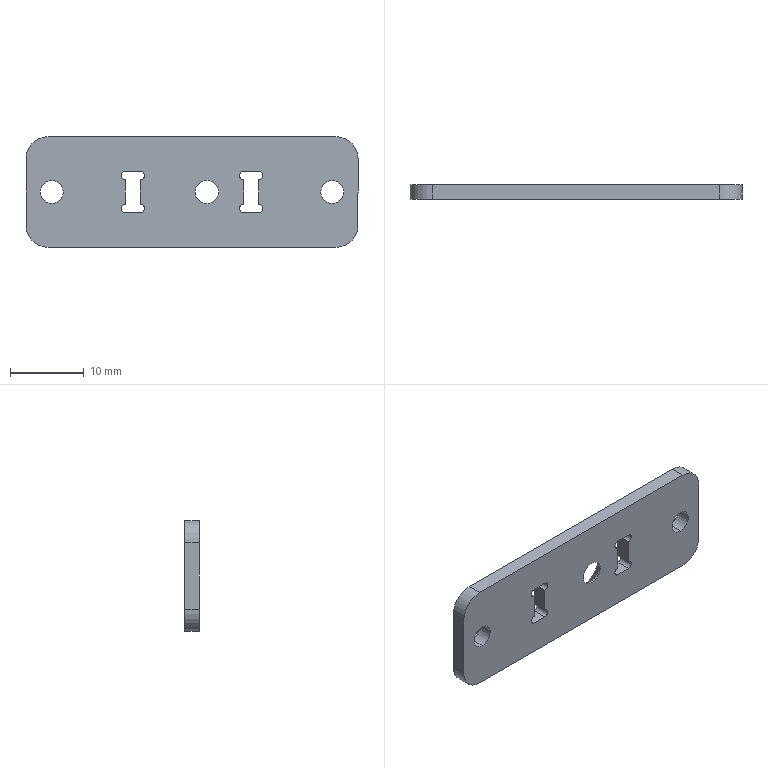Part | SolidWorks | features Extrusion 1, Fillet 1, HoleWzd 1 | 1 solid | 34 faces | box 45 x 2 x 15 mm | volume 1215 mm3 | cylinder 18 | plane 14 | cone 2 | commonest cylinder face diameters 1.1 x8 3.1 x4 6 x4 3.2 x2
STEP:
#1=CARTESIAN_POINT('',(2.025,0.3,-1.6));
#2=VERTEX_POINT('',#1);
#3=CARTESIAN_POINT('',(2.025,0.3,1.6));
#4=VERTEX_POINT('',#3);
#5=CARTESIAN_POINT('',(2.025,0.3,0.));
#6=DIRECTION('',(0.,1.,0.));
#7=DIRECTION('',(0.,0.,1.));
#8=AXIS2_PLACEMENT_3D('',#5,#6,#7);
#9=CIRCLE('',#8,1.6);
#10=EDGE_CURVE('',#2,#4,#9,.T.);
#11=ORIENTED_EDGE('',*,*,#10,.F.);
#12=CARTESIAN_POINT('',(2.025,2.,-3.3));
#13=VERTEX_POINT('',#12);
#14=CARTESIAN_POINT('',(2.025,2.,-3.3));
#15=DIRECTION('',(0.,0.7071,-0.7071));
#16=VECTOR('',#15,1000.);
#17=LINE('',#14,#16);
#18=EDGE_CURVE('',#2,#13,#17,.T.);
#19=ORIENTED_EDGE('',*,*,#18,.T.);
#20=CARTESIAN_POINT('',(2.025,2.,3.3));
#21=VERTEX_POINT('',#20);
#22=CARTESIAN_POINT('',(2.025,2.,0.));
#23=DIRECTION('',(0.,1.,0.));
#24=DIRECTION('',(0.,0.,1.));
#25=AXIS2_PLACEMENT_3D('',#22,#23,#24);
#26=CIRCLE('',#25,3.3);
#27=EDGE_CURVE('',#13,#21,#26,.T.);
#28=ORIENTED_EDGE('',*,*,#27,.T.);
#29=CARTESIAN_POINT('',(2.025,2.,3.3));
#30=DIRECTION('',(0.,0.7071,0.7071));
#31=VECTOR('',#30,1000.);
#32=LINE('',#29,#31);
#33=EDGE_CURVE('',#4,#21,#32,.T.);
#34=ORIENTED_EDGE('',*,*,#33,.F.);
#35=EDGE_LOOP('',(#11,#19,#28,#34));
#36=FACE_OUTER_BOUND('',#35,.T.);
#37=CARTESIAN_POINT('',(2.025,2.,0.));
#38=DIRECTION('',(0.,1.,0.));
#39=DIRECTION('',(0.,0.,1.));
#40=AXIS2_PLACEMENT_3D('',#37,#38,#39);
#41=CONICAL_SURFACE('',#40,3.3,0.7854);
#42=ADVANCED_FACE('',(#36),#41,.F.);
#43=CARTESIAN_POINT('',(2.025,0.,-1.6));
#44=VERTEX_POINT('',#43);
#45=CARTESIAN_POINT('',(2.025,0.,1.6));
#46=VERTEX_POINT('',#45);
#47=CARTESIAN_POINT('',(2.025,0.,0.));
#48=DIRECTION('',(0.,1.,0.));
#49=DIRECTION('',(0.,0.,1.));
#50=AXIS2_PLACEMENT_3D('',#47,#48,#49);
#51=CIRCLE('',#50,1.6);
#52=EDGE_CURVE('',#44,#46,#51,.T.);
#53=ORIENTED_EDGE('',*,*,#52,.F.);
#54=CARTESIAN_POINT('',(2.025,2.,-1.6));
#55=DIRECTION('',(0.,1.,0.));
#56=VECTOR('',#55,1000.);
#57=LINE('',#54,#56);
#58=EDGE_CURVE('',#44,#2,#57,.T.);
#59=ORIENTED_EDGE('',*,*,#58,.T.);
#60=ORIENTED_EDGE('',*,*,#10,.T.);
#61=CARTESIAN_POINT('',(2.025,2.,1.6));
#62=DIRECTION('',(0.,1.,0.));
#63=VECTOR('',#62,1000.);
#64=LINE('',#61,#63);
#65=EDGE_CURVE('',#46,#4,#64,.T.);
#66=ORIENTED_EDGE('',*,*,#65,.F.);
#67=EDGE_LOOP('',(#53,#59,#60,#66));
#68=FACE_OUTER_BOUND('',#67,.T.);
#69=CARTESIAN_POINT('',(2.025,2.,0.));
#70=DIRECTION('',(0.,1.,0.));
#71=DIRECTION('',(0.,0.,1.));
#72=AXIS2_PLACEMENT_3D('',#69,#70,#71);
#73=CYLINDRICAL_SURFACE('',#72,1.6);
#74=ADVANCED_FACE('',(#68),#73,.F.);
#75=CARTESIAN_POINT('',(19.,2.,-1.55));
#76=VERTEX_POINT('',#75);
#77=CARTESIAN_POINT('',(19.,2.,1.55));
#78=VERTEX_POINT('',#77);
#79=CARTESIAN_POINT('',(19.,2.,0.));
#80=DIRECTION('',(0.,1.,0.));
#81=DIRECTION('',(0.,0.,1.));
#82=AXIS2_PLACEMENT_3D('',#79,#80,#81);
#83=CIRCLE('',#82,1.55);
#84=EDGE_CURVE('',#76,#78,#83,.T.);
#85=ORIENTED_EDGE('',*,*,#84,.T.);
#86=CARTESIAN_POINT('',(19.,0.,1.55));
#87=VERTEX_POINT('',#86);
#88=CARTESIAN_POINT('',(19.,2.,1.55));
#89=DIRECTION('',(0.,-1.,0.));
#90=VECTOR('',#89,1000.);
#91=LINE('',#88,#90);
#92=EDGE_CURVE('',#78,#87,#91,.T.);
#93=ORIENTED_EDGE('',*,*,#92,.T.);
#94=CARTESIAN_POINT('',(19.,0.,-1.55));
#95=VERTEX_POINT('',#94);
#96=CARTESIAN_POINT('',(19.,0.,0.));
#97=DIRECTION('',(0.,1.,0.));
#98=DIRECTION('',(0.,0.,1.));
#99=AXIS2_PLACEMENT_3D('',#96,#97,#98);
#100=CIRCLE('',#99,1.55);
#101=EDGE_CURVE('',#95,#87,#100,.T.);
#102=ORIENTED_EDGE('',*,*,#101,.F.);
#103=CARTESIAN_POINT('',(19.,2.,-1.55));
#104=DIRECTION('',(0.,-1.,0.));
#105=VECTOR('',#104,1000.);
#106=LINE('',#103,#105);
#107=EDGE_CURVE('',#76,#95,#106,.T.);
#108=ORIENTED_EDGE('',*,*,#107,.F.);
#109=EDGE_LOOP('',(#85,#93,#102,#108));
#110=FACE_OUTER_BOUND('',#109,.T.);
#111=CARTESIAN_POINT('',(19.,2.,0.));
#112=DIRECTION('',(0.,-1.,0.));
#113=DIRECTION('',(0.,0.,-1.));
#114=AXIS2_PLACEMENT_3D('',#111,#112,#113);
#115=CYLINDRICAL_SURFACE('',#114,1.55);
#116=ADVANCED_FACE('',(#110),#115,.F.);
#117=CARTESIAN_POINT('',(-19.,2.,1.55));
#118=VERTEX_POINT('',#117);
#119=CARTESIAN_POINT('',(-19.,2.,-1.55));
#120=VERTEX_POINT('',#119);
#121=CARTESIAN_POINT('',(-19.,2.,0.));
#122=DIRECTION('',(0.,-1.,0.));
#123=DIRECTION('',(0.,0.,1.));
#124=AXIS2_PLACEMENT_3D('',#121,#122,#123);
#125=CIRCLE('',#124,1.55);
#126=EDGE_CURVE('',#118,#120,#125,.T.);
#127=ORIENTED_EDGE('',*,*,#126,.F.);
#128=CARTESIAN_POINT('',(-19.,0.,1.55));
#129=VERTEX_POINT('',#128);
#130=CARTESIAN_POINT('',(-19.,2.,1.55));
#131=DIRECTION('',(0.,-1.,0.));
#132=VECTOR('',#131,1000.);
#133=LINE('',#130,#132);
#134=EDGE_CURVE('',#118,#129,#133,.T.);
#135=ORIENTED_EDGE('',*,*,#134,.T.);
#136=CARTESIAN_POINT('',(-19.,0.,-1.55));
#137=VERTEX_POINT('',#136);
#138=CARTESIAN_POINT('',(-19.,0.,0.));
#139=DIRECTION('',(0.,-1.,0.));
#140=DIRECTION('',(0.,0.,1.));
#141=AXIS2_PLACEMENT_3D('',#138,#139,#140);
#142=CIRCLE('',#141,1.55);
#143=EDGE_CURVE('',#129,#137,#142,.T.);
#144=ORIENTED_EDGE('',*,*,#143,.T.);
#145=CARTESIAN_POINT('',(-19.,2.,-1.55));
#146=DIRECTION('',(0.,-1.,0.));
#147=VECTOR('',#146,1000.);
#148=LINE('',#145,#147);
#149=EDGE_CURVE('',#120,#137,#148,.T.);
#150=ORIENTED_EDGE('',*,*,#149,.F.);
#151=EDGE_LOOP('',(#127,#135,#144,#150));
#152=FACE_OUTER_BOUND('',#151,.T.);
#153=CARTESIAN_POINT('',(-19.,2.,0.));
#154=DIRECTION('',(0.,-1.,0.));
#155=DIRECTION('',(0.,0.,-1.));
#156=AXIS2_PLACEMENT_3D('',#153,#154,#155);
#157=CYLINDRICAL_SURFACE('',#156,1.55);
#158=ADVANCED_FACE('',(#152),#157,.F.);
#159=CARTESIAN_POINT('',(-9.05,0.,-1.675));
#160=VERTEX_POINT('',#159);
#161=CARTESIAN_POINT('',(-9.05,0.,1.675));
#162=VERTEX_POINT('',#161);
#163=CARTESIAN_POINT('',(-9.05,0.,0.));
#164=DIRECTION('',(0.,0.,1.));
#165=VECTOR('',#164,1000.);
#166=LINE('',#163,#165);
#167=EDGE_CURVE('',#160,#162,#166,.T.);
#168=ORIENTED_EDGE('',*,*,#167,.F.);
#169=CARTESIAN_POINT('',(-9.05,2.,-1.675));
#170=VERTEX_POINT('',#169);
#171=CARTESIAN_POINT('',(-9.05,2.,-1.675));
#172=DIRECTION('',(0.,-1.,0.));
#173=VECTOR('',#172,1000.);
#174=LINE('',#171,#173);
#175=EDGE_CURVE('',#170,#160,#174,.T.);
#176=ORIENTED_EDGE('',*,*,#175,.F.);
#177=CARTESIAN_POINT('',(-9.05,2.,1.675));
#178=VERTEX_POINT('',#177);
#179=CARTESIAN_POINT('',(-9.05,2.,0.));
#180=DIRECTION('',(0.,0.,1.));
#181=VECTOR('',#180,1000.);
#182=LINE('',#179,#181);
#183=EDGE_CURVE('',#170,#178,#182,.T.);
#184=ORIENTED_EDGE('',*,*,#183,.T.);
#185=CARTESIAN_POINT('',(-9.05,2.,1.675));
#186=DIRECTION('',(0.,-1.,0.));
#187=VECTOR('',#186,1000.);
#188=LINE('',#185,#187);
#189=EDGE_CURVE('',#178,#162,#188,.T.);
#190=ORIENTED_EDGE('',*,*,#189,.T.);
#191=EDGE_LOOP('',(#168,#176,#184,#190));
#192=FACE_OUTER_BOUND('',#191,.T.);
#193=CARTESIAN_POINT('',(-9.05,2.,0.));
#194=DIRECTION('',(1.,0.,0.));
#195=DIRECTION('',(0.,0.,-1.));
#196=AXIS2_PLACEMENT_3D('',#193,#194,#195);
#197=PLANE('',#196);
#198=ADVANCED_FACE('',(#192),#197,.T.);
#199=CARTESIAN_POINT('',(-9.05,0.,-2.775));
#200=VERTEX_POINT('',#199);
#201=CARTESIAN_POINT('',(-9.05,0.,-2.225));
#202=DIRECTION('',(0.,-1.,0.));
#203=DIRECTION('',(0.,0.,1.));
#204=AXIS2_PLACEMENT_3D('',#201,#202,#203);
#205=CIRCLE('',#204,0.55);
#206=EDGE_CURVE('',#160,#200,#205,.T.);
#207=ORIENTED_EDGE('',*,*,#206,.T.);
#208=CARTESIAN_POINT('',(-9.05,2.,-2.775));
#209=VERTEX_POINT('',#208);
#210=CARTESIAN_POINT('',(-9.05,2.,-2.775));
#211=DIRECTION('',(0.,-1.,0.));
#212=VECTOR('',#211,1000.);
#213=LINE('',#210,#212);
#214=EDGE_CURVE('',#209,#200,#213,.T.);
#215=ORIENTED_EDGE('',*,*,#214,.F.);
#216=CARTESIAN_POINT('',(-9.05,2.,-2.225));
#217=DIRECTION('',(0.,-1.,0.));
#218=DIRECTION('',(0.,0.,1.));
#219=AXIS2_PLACEMENT_3D('',#216,#217,#218);
#220=CIRCLE('',#219,0.55);
#221=EDGE_CURVE('',#170,#209,#220,.T.);
#222=ORIENTED_EDGE('',*,*,#221,.F.);
#223=ORIENTED_EDGE('',*,*,#175,.T.);
#224=EDGE_LOOP('',(#207,#215,#222,#223));
#225=FACE_OUTER_BOUND('',#224,.T.);
#226=CARTESIAN_POINT('',(-9.05,2.,-2.225));
#227=DIRECTION('',(0.,-1.,0.));
#228=DIRECTION('',(0.,0.,-1.));
#229=AXIS2_PLACEMENT_3D('',#226,#227,#228);
#230=CYLINDRICAL_SURFACE('',#229,0.55);
#231=ADVANCED_FACE('',(#225),#230,.F.);
#232=CARTESIAN_POINT('',(-7.,0.,-2.775));
#233=VERTEX_POINT('',#232);
#234=CARTESIAN_POINT('',(0.,0.,-2.775));
#235=DIRECTION('',(-1.,0.,0.));
#236=VECTOR('',#235,1000.);
#237=LINE('',#234,#236);
#238=EDGE_CURVE('',#233,#200,#237,.T.);
#239=ORIENTED_EDGE('',*,*,#238,.F.);
#240=CARTESIAN_POINT('',(-7.,2.,-2.775));
#241=VERTEX_POINT('',#240);
#242=CARTESIAN_POINT('',(-7.,2.,-2.775));
#243=DIRECTION('',(0.,-1.,0.));
#244=VECTOR('',#243,1000.);
#245=LINE('',#242,#244);
#246=EDGE_CURVE('',#241,#233,#245,.T.);
#247=ORIENTED_EDGE('',*,*,#246,.F.);
#248=CARTESIAN_POINT('',(0.,2.,-2.775));
#249=DIRECTION('',(-1.,0.,0.));
#250=VECTOR('',#249,1000.);
#251=LINE('',#248,#250);
#252=EDGE_CURVE('',#241,#209,#251,.T.);
#253=ORIENTED_EDGE('',*,*,#252,.T.);
#254=ORIENTED_EDGE('',*,*,#214,.T.);
#255=EDGE_LOOP('',(#239,#247,#253,#254));
#256=FACE_OUTER_BOUND('',#255,.T.);
#257=CARTESIAN_POINT('',(0.,2.,-2.775));
#258=DIRECTION('',(0.,0.,1.));
#259=DIRECTION('',(1.,0.,0.));
#260=AXIS2_PLACEMENT_3D('',#257,#258,#259);
#261=PLANE('',#260);
#262=ADVANCED_FACE('',(#256),#261,.T.);
#263=CARTESIAN_POINT('',(-7.,0.,-1.675));
#264=VERTEX_POINT('',#263);
#265=CARTESIAN_POINT('',(-7.,0.,-2.225));
#266=DIRECTION('',(0.,1.,0.));
#267=DIRECTION('',(0.,0.,1.));
#268=AXIS2_PLACEMENT_3D('',#265,#266,#267);
#269=CIRCLE('',#268,0.55);
#270=EDGE_CURVE('',#264,#233,#269,.T.);
#271=ORIENTED_EDGE('',*,*,#270,.F.);
#272=CARTESIAN_POINT('',(-7.,2.,-1.675));
#273=VERTEX_POINT('',#272);
#274=CARTESIAN_POINT('',(-7.,2.,-1.675));
#275=DIRECTION('',(0.,-1.,0.));
#276=VECTOR('',#275,1000.);
#277=LINE('',#274,#276);
#278=EDGE_CURVE('',#273,#264,#277,.T.);
#279=ORIENTED_EDGE('',*,*,#278,.F.);
#280=CARTESIAN_POINT('',(-7.,2.,-2.225));
#281=DIRECTION('',(0.,1.,0.));
#282=DIRECTION('',(0.,0.,1.));
#283=AXIS2_PLACEMENT_3D('',#280,#281,#282);
#284=CIRCLE('',#283,0.55);
#285=EDGE_CURVE('',#273,#241,#284,.T.);
#286=ORIENTED_EDGE('',*,*,#285,.T.);
#287=ORIENTED_EDGE('',*,*,#246,.T.);
#288=EDGE_LOOP('',(#271,#279,#286,#287));
#289=FACE_OUTER_BOUND('',#288,.T.);
#290=CARTESIAN_POINT('',(-7.,2.,-2.225));
#291=DIRECTION('',(0.,-1.,0.));
#292=DIRECTION('',(0.,0.,-1.));
#293=AXIS2_PLACEMENT_3D('',#290,#291,#292);
#294=CYLINDRICAL_SURFACE('',#293,0.55);
#295=ADVANCED_FACE('',(#289),#294,.F.);
#296=CARTESIAN_POINT('',(-7.,0.,1.675));
#297=VERTEX_POINT('',#296);
#298=CARTESIAN_POINT('',(-7.,0.,0.));
#299=DIRECTION('',(0.,0.,1.));
#300=VECTOR('',#299,1000.);
#301=LINE('',#298,#300);
#302=EDGE_CURVE('',#264,#297,#301,.T.);
#303=ORIENTED_EDGE('',*,*,#302,.T.);
#304=CARTESIAN_POINT('',(-7.,2.,1.675));
#305=VERTEX_POINT('',#304);
#306=CARTESIAN_POINT('',(-7.,2.,1.675));
#307=DIRECTION('',(0.,-1.,0.));
#308=VECTOR('',#307,1000.);
#309=LINE('',#306,#308);
#310=EDGE_CURVE('',#305,#297,#309,.T.);
#311=ORIENTED_EDGE('',*,*,#310,.F.);
#312=CARTESIAN_POINT('',(-7.,2.,0.));
#313=DIRECTION('',(0.,0.,1.));
#314=VECTOR('',#313,1000.);
#315=LINE('',#312,#314);
#316=EDGE_CURVE('',#273,#305,#315,.T.);
#317=ORIENTED_EDGE('',*,*,#316,.F.);
#318=ORIENTED_EDGE('',*,*,#278,.T.);
#319=EDGE_LOOP('',(#303,#311,#317,#318));
#320=FACE_OUTER_BOUND('',#319,.T.);
#321=CARTESIAN_POINT('',(-7.,2.,0.));
#322=DIRECTION('',(1.,0.,0.));
#323=DIRECTION('',(0.,0.,-1.));
#324=AXIS2_PLACEMENT_3D('',#321,#322,#323);
#325=PLANE('',#324);
#326=ADVANCED_FACE('',(#320),#325,.F.);
#327=CARTESIAN_POINT('',(-7.,0.,2.775));
#328=VERTEX_POINT('',#327);
#329=CARTESIAN_POINT('',(-7.,0.,2.225));
#330=DIRECTION('',(0.,-1.,0.));
#331=DIRECTION('',(0.,0.,1.));
#332=AXIS2_PLACEMENT_3D('',#329,#330,#331);
#333=CIRCLE('',#332,0.55);
#334=EDGE_CURVE('',#297,#328,#333,.T.);
#335=ORIENTED_EDGE('',*,*,#334,.T.);
#336=CARTESIAN_POINT('',(-7.,2.,2.775));
#337=VERTEX_POINT('',#336);
#338=CARTESIAN_POINT('',(-7.,2.,2.775));
#339=DIRECTION('',(0.,-1.,0.));
#340=VECTOR('',#339,1000.);
#341=LINE('',#338,#340);
#342=EDGE_CURVE('',#337,#328,#341,.T.);
#343=ORIENTED_EDGE('',*,*,#342,.F.);
#344=CARTESIAN_POINT('',(-7.,2.,2.225));
#345=DIRECTION('',(0.,-1.,0.));
#346=DIRECTION('',(0.,0.,1.));
#347=AXIS2_PLACEMENT_3D('',#344,#345,#346);
#348=CIRCLE('',#347,0.55);
#349=EDGE_CURVE('',#305,#337,#348,.T.);
#350=ORIENTED_EDGE('',*,*,#349,.F.);
#351=ORIENTED_EDGE('',*,*,#310,.T.);
#352=EDGE_LOOP('',(#335,#343,#350,#351));
#353=FACE_OUTER_BOUND('',#352,.T.);
#354=CARTESIAN_POINT('',(-7.,2.,2.225));
#355=DIRECTION('',(0.,-1.,0.));
#356=DIRECTION('',(0.,0.,-1.));
#357=AXIS2_PLACEMENT_3D('',#354,#355,#356);
#358=CYLINDRICAL_SURFACE('',#357,0.55);
#359=ADVANCED_FACE('',(#353),#358,.F.);
#360=CARTESIAN_POINT('',(-9.05,0.,2.775));
#361=VERTEX_POINT('',#360);
#362=CARTESIAN_POINT('',(0.,0.,2.775));
#363=DIRECTION('',(-1.,0.,0.));
#364=VECTOR('',#363,1000.);
#365=LINE('',#362,#364);
#366=EDGE_CURVE('',#328,#361,#365,.T.);
#367=ORIENTED_EDGE('',*,*,#366,.T.);
#368=CARTESIAN_POINT('',(-9.05,2.,2.775));
#369=VERTEX_POINT('',#368);
#370=CARTESIAN_POINT('',(-9.05,2.,2.775));
#371=DIRECTION('',(0.,-1.,0.));
#372=VECTOR('',#371,1000.);
#373=LINE('',#370,#372);
#374=EDGE_CURVE('',#369,#361,#373,.T.);
#375=ORIENTED_EDGE('',*,*,#374,.F.);
#376=CARTESIAN_POINT('',(0.,2.,2.775));
#377=DIRECTION('',(-1.,0.,0.));
#378=VECTOR('',#377,1000.);
#379=LINE('',#376,#378);
#380=EDGE_CURVE('',#337,#369,#379,.T.);
#381=ORIENTED_EDGE('',*,*,#380,.F.);
#382=ORIENTED_EDGE('',*,*,#342,.T.);
#383=EDGE_LOOP('',(#367,#375,#381,#382));
#384=FACE_OUTER_BOUND('',#383,.T.);
#385=CARTESIAN_POINT('',(0.,2.,2.775));
#386=DIRECTION('',(0.,0.,1.));
#387=DIRECTION('',(1.,0.,0.));
#388=AXIS2_PLACEMENT_3D('',#385,#386,#387);
#389=PLANE('',#388);
#390=ADVANCED_FACE('',(#384),#389,.F.);
#391=CARTESIAN_POINT('',(22.5,2.,-4.5));
#392=VERTEX_POINT('',#391);
#393=CARTESIAN_POINT('',(22.5,2.,4.5));
#394=VERTEX_POINT('',#393);
#395=CARTESIAN_POINT('',(22.5,2.,0.));
#396=DIRECTION('',(0.,0.,1.));
#397=VECTOR('',#396,1000.);
#398=LINE('',#395,#397);
#399=EDGE_CURVE('',#392,#394,#398,.T.);
#400=ORIENTED_EDGE('',*,*,#399,.T.);
#401=CARTESIAN_POINT('',(22.5,0.,4.5));
#402=VERTEX_POINT('',#401);
#403=CARTESIAN_POINT('',(22.5,0.,4.5));
#404=DIRECTION('',(0.,-1.,0.));
#405=VECTOR('',#404,1000.);
#406=LINE('',#403,#405);
#407=EDGE_CURVE('',#394,#402,#406,.T.);
#408=ORIENTED_EDGE('',*,*,#407,.T.);
#409=CARTESIAN_POINT('',(22.5,0.,-4.5));
#410=VERTEX_POINT('',#409);
#411=CARTESIAN_POINT('',(22.5,0.,0.));
#412=DIRECTION('',(0.,0.,1.));
#413=VECTOR('',#412,1000.);
#414=LINE('',#411,#413);
#415=EDGE_CURVE('',#410,#402,#414,.T.);
#416=ORIENTED_EDGE('',*,*,#415,.F.);
#417=CARTESIAN_POINT('',(22.5,2.,-4.5));
#418=DIRECTION('',(0.,1.,0.));
#419=VECTOR('',#418,1000.);
#420=LINE('',#417,#419);
#421=EDGE_CURVE('',#410,#392,#420,.T.);
#422=ORIENTED_EDGE('',*,*,#421,.T.);
#423=EDGE_LOOP('',(#400,#408,#416,#422));
#424=FACE_OUTER_BOUND('',#423,.T.);
#425=CARTESIAN_POINT('',(22.5,2.,0.));
#426=DIRECTION('',(1.,0.,0.));
#427=DIRECTION('',(0.,0.,-1.));
#428=AXIS2_PLACEMENT_3D('',#425,#426,#427);
#429=PLANE('',#428);
#430=ADVANCED_FACE('',(#424),#429,.T.);
#431=CARTESIAN_POINT('',(-19.5,2.,-7.5));
#432=VERTEX_POINT('',#431);
#433=CARTESIAN_POINT('',(19.5,2.,-7.5));
#434=VERTEX_POINT('',#433);
#435=CARTESIAN_POINT('',(0.,2.,-7.5));
#436=DIRECTION('',(1.,0.,0.));
#437=VECTOR('',#436,1000.);
#438=LINE('',#435,#437);
#439=EDGE_CURVE('',#432,#434,#438,.T.);
#440=ORIENTED_EDGE('',*,*,#439,.T.);
#441=CARTESIAN_POINT('',(19.5,0.,-7.5));
#442=VERTEX_POINT('',#441);
#443=CARTESIAN_POINT('',(19.5,2.,-7.5));
#444=DIRECTION('',(0.,-1.,0.));
#445=VECTOR('',#444,1000.);
#446=LINE('',#443,#445);
#447=EDGE_CURVE('',#434,#442,#446,.T.);
#448=ORIENTED_EDGE('',*,*,#447,.T.);
#449=CARTESIAN_POINT('',(-19.5,0.,-7.5));
#450=VERTEX_POINT('',#449);
#451=CARTESIAN_POINT('',(0.,0.,-7.5));
#452=DIRECTION('',(1.,0.,0.));
#453=VECTOR('',#452,1000.);
#454=LINE('',#451,#453);
#455=EDGE_CURVE('',#450,#442,#454,.T.);
#456=ORIENTED_EDGE('',*,*,#455,.F.);
#457=CARTESIAN_POINT('',(-19.5,2.,-7.5));
#458=DIRECTION('',(0.,1.,0.));
#459=VECTOR('',#458,1000.);
#460=LINE('',#457,#459);
#461=EDGE_CURVE('',#450,#432,#460,.T.);
#462=ORIENTED_EDGE('',*,*,#461,.T.);
#463=EDGE_LOOP('',(#440,#448,#456,#462));
#464=FACE_OUTER_BOUND('',#463,.T.);
#465=CARTESIAN_POINT('',(0.,2.,-7.5));
#466=DIRECTION('',(0.,0.,-1.));
#467=DIRECTION('',(-1.,0.,0.));
#468=AXIS2_PLACEMENT_3D('',#465,#466,#467);
#469=PLANE('',#468);
#470=ADVANCED_FACE('',(#464),#469,.T.);
#471=CARTESIAN_POINT('',(-22.5,0.,-4.5));
#472=VERTEX_POINT('',#471);
#473=CARTESIAN_POINT('',(-22.5,0.,4.5));
#474=VERTEX_POINT('',#473);
#475=CARTESIAN_POINT('',(-22.5,0.,0.));
#476=DIRECTION('',(0.,0.,1.));
#477=VECTOR('',#476,1000.);
#478=LINE('',#475,#477);
#479=EDGE_CURVE('',#472,#474,#478,.T.);
#480=ORIENTED_EDGE('',*,*,#479,.T.);
#481=CARTESIAN_POINT('',(-22.5,2.,4.5));
#482=VERTEX_POINT('',#481);
#483=CARTESIAN_POINT('',(-22.5,2.,4.5));
#484=DIRECTION('',(0.,1.,0.));
#485=VECTOR('',#484,1000.);
#486=LINE('',#483,#485);
#487=EDGE_CURVE('',#474,#482,#486,.T.);
#488=ORIENTED_EDGE('',*,*,#487,.T.);
#489=CARTESIAN_POINT('',(-22.5,2.,-4.5));
#490=VERTEX_POINT('',#489);
#491=CARTESIAN_POINT('',(-22.5,2.,0.));
#492=DIRECTION('',(0.,0.,1.));
#493=VECTOR('',#492,1000.);
#494=LINE('',#491,#493);
#495=EDGE_CURVE('',#490,#482,#494,.T.);
#496=ORIENTED_EDGE('',*,*,#495,.F.);
#497=CARTESIAN_POINT('',(-22.5,0.,-4.5));
#498=DIRECTION('',(0.,-1.,0.));
#499=VECTOR('',#498,1000.);
#500=LINE('',#497,#499);
#501=EDGE_CURVE('',#490,#472,#500,.T.);
#502=ORIENTED_EDGE('',*,*,#501,.T.);
#503=EDGE_LOOP('',(#480,#488,#496,#502));
#504=FACE_OUTER_BOUND('',#503,.T.);
#505=CARTESIAN_POINT('',(-22.5,2.,0.));
#506=DIRECTION('',(1.,0.,0.));
#507=DIRECTION('',(0.,0.,-1.));
#508=AXIS2_PLACEMENT_3D('',#505,#506,#507);
#509=PLANE('',#508);
#510=ADVANCED_FACE('',(#504),#509,.F.);
#511=CARTESIAN_POINT('',(7.,0.,1.675));
#512=VERTEX_POINT('',#511);
#513=CARTESIAN_POINT('',(7.,0.,2.775));
#514=VERTEX_POINT('',#513);
#515=CARTESIAN_POINT('',(7.,0.,2.225));
#516=DIRECTION('',(0.,1.,0.));
#517=DIRECTION('',(0.,0.,1.));
#518=AXIS2_PLACEMENT_3D('',#515,#516,#517);
#519=CIRCLE('',#518,0.55);
#520=EDGE_CURVE('',#512,#514,#519,.T.);
#521=ORIENTED_EDGE('',*,*,#520,.F.);
#522=CARTESIAN_POINT('',(7.,2.,1.675));
#523=VERTEX_POINT('',#522);
#524=CARTESIAN_POINT('',(7.,2.,1.675));
#525=DIRECTION('',(0.,-1.,0.));
#526=VECTOR('',#525,1000.);
#527=LINE('',#524,#526);
#528=EDGE_CURVE('',#523,#512,#527,.T.);
#529=ORIENTED_EDGE('',*,*,#528,.F.);
#530=CARTESIAN_POINT('',(7.,2.,2.775));
#531=VERTEX_POINT('',#530);
#532=CARTESIAN_POINT('',(7.,2.,2.225));
#533=DIRECTION('',(0.,1.,0.));
#534=DIRECTION('',(0.,0.,1.));
#535=AXIS2_PLACEMENT_3D('',#532,#533,#534);
#536=CIRCLE('',#535,0.55);
#537=EDGE_CURVE('',#523,#531,#536,.T.);
#538=ORIENTED_EDGE('',*,*,#537,.T.);
#539=CARTESIAN_POINT('',(7.,2.,2.775));
#540=DIRECTION('',(0.,-1.,0.));
#541=VECTOR('',#540,1000.);
#542=LINE('',#539,#541);
#543=EDGE_CURVE('',#531,#514,#542,.T.);
#544=ORIENTED_EDGE('',*,*,#543,.T.);
#545=EDGE_LOOP('',(#521,#529,#538,#544));
#546=FACE_OUTER_BOUND('',#545,.T.);
#547=CARTESIAN_POINT('',(7.,2.,2.225));
#548=DIRECTION('',(0.,-1.,0.));
#549=DIRECTION('',(0.,0.,-1.));
#550=AXIS2_PLACEMENT_3D('',#547,#548,#549);
#551=CYLINDRICAL_SURFACE('',#550,0.55);
#552=ADVANCED_FACE('',(#546),#551,.F.);
#553=CARTESIAN_POINT('',(7.,0.,-1.675));
#554=VERTEX_POINT('',#553);
#555=CARTESIAN_POINT('',(7.,0.,0.));
#556=DIRECTION('',(0.,0.,1.));
#557=VECTOR('',#556,1000.);
#558=LINE('',#555,#557);
#559=EDGE_CURVE('',#554,#512,#558,.T.);
#560=ORIENTED_EDGE('',*,*,#559,.F.);
#561=CARTESIAN_POINT('',(7.,2.,-1.675));
#562=VERTEX_POINT('',#561);
#563=CARTESIAN_POINT('',(7.,2.,-1.675));
#564=DIRECTION('',(0.,-1.,0.));
#565=VECTOR('',#564,1000.);
#566=LINE('',#563,#565);
#567=EDGE_CURVE('',#562,#554,#566,.T.);
#568=ORIENTED_EDGE('',*,*,#567,.F.);
#569=CARTESIAN_POINT('',(7.,2.,0.));
#570=DIRECTION('',(0.,0.,1.));
#571=VECTOR('',#570,1000.);
#572=LINE('',#569,#571);
#573=EDGE_CURVE('',#562,#523,#572,.T.);
#574=ORIENTED_EDGE('',*,*,#573,.T.);
#575=ORIENTED_EDGE('',*,*,#528,.T.);
#576=EDGE_LOOP('',(#560,#568,#574,#575));
#577=FACE_OUTER_BOUND('',#576,.T.);
#578=CARTESIAN_POINT('',(7.,2.,0.));
#579=DIRECTION('',(1.,0.,0.));
#580=DIRECTION('',(0.,0.,-1.));
#581=AXIS2_PLACEMENT_3D('',#578,#579,#580);
#582=PLANE('',#581);
#583=ADVANCED_FACE('',(#577),#582,.T.);
#584=CARTESIAN_POINT('',(7.,0.,-2.775));
#585=VERTEX_POINT('',#584);
#586=CARTESIAN_POINT('',(7.,0.,-2.225));
#587=DIRECTION('',(0.,-1.,0.));
#588=DIRECTION('',(0.,0.,1.));
#589=AXIS2_PLACEMENT_3D('',#586,#587,#588);
#590=CIRCLE('',#589,0.55);
#591=EDGE_CURVE('',#554,#585,#590,.T.);
#592=ORIENTED_EDGE('',*,*,#591,.T.);
#593=CARTESIAN_POINT('',(7.,2.,-2.775));
#594=VERTEX_POINT('',#593);
#595=CARTESIAN_POINT('',(7.,2.,-2.775));
#596=DIRECTION('',(0.,-1.,0.));
#597=VECTOR('',#596,1000.);
#598=LINE('',#595,#597);
#599=EDGE_CURVE('',#594,#585,#598,.T.);
#600=ORIENTED_EDGE('',*,*,#599,.F.);
#601=CARTESIAN_POINT('',(7.,2.,-2.225));
#602=DIRECTION('',(0.,-1.,0.));
#603=DIRECTION('',(0.,0.,1.));
#604=AXIS2_PLACEMENT_3D('',#601,#602,#603);
#605=CIRCLE('',#604,0.55);
#606=EDGE_CURVE('',#562,#594,#605,.T.);
#607=ORIENTED_EDGE('',*,*,#606,.F.);
#608=ORIENTED_EDGE('',*,*,#567,.T.);
#609=EDGE_LOOP('',(#592,#600,#607,#608));
#610=FACE_OUTER_BOUND('',#609,.T.);
#611=CARTESIAN_POINT('',(7.,2.,-2.225));
#612=DIRECTION('',(0.,-1.,0.));
#613=DIRECTION('',(0.,0.,-1.));
#614=AXIS2_PLACEMENT_3D('',#611,#612,#613);
#615=CYLINDRICAL_SURFACE('',#614,0.55);
#616=ADVANCED_FACE('',(#610),#615,.F.);
#617=CARTESIAN_POINT('',(9.05,0.,-2.775));
#618=VERTEX_POINT('',#617);
#619=CARTESIAN_POINT('',(0.,0.,-2.775));
#620=DIRECTION('',(1.,0.,0.));
#621=VECTOR('',#620,1000.);
#622=LINE('',#619,#621);
#623=EDGE_CURVE('',#585,#618,#622,.T.);
#624=ORIENTED_EDGE('',*,*,#623,.T.);
#625=CARTESIAN_POINT('',(9.05,2.,-2.775));
#626=VERTEX_POINT('',#625);
#627=CARTESIAN_POINT('',(9.05,2.,-2.775));
#628=DIRECTION('',(0.,-1.,0.));
#629=VECTOR('',#628,1000.);
#630=LINE('',#627,#629);
#631=EDGE_CURVE('',#626,#618,#630,.T.);
#632=ORIENTED_EDGE('',*,*,#631,.F.);
#633=CARTESIAN_POINT('',(0.,2.,-2.775));
#634=DIRECTION('',(1.,0.,0.));
#635=VECTOR('',#634,1000.);
#636=LINE('',#633,#635);
#637=EDGE_CURVE('',#594,#626,#636,.T.);
#638=ORIENTED_EDGE('',*,*,#637,.F.);
#639=ORIENTED_EDGE('',*,*,#599,.T.);
#640=EDGE_LOOP('',(#624,#632,#638,#639));
#641=FACE_OUTER_BOUND('',#640,.T.);
#642=CARTESIAN_POINT('',(0.,2.,-2.775));
#643=DIRECTION('',(0.,0.,-1.));
#644=DIRECTION('',(-1.,0.,0.));
#645=AXIS2_PLACEMENT_3D('',#642,#643,#644);
#646=PLANE('',#645);
#647=ADVANCED_FACE('',(#641),#646,.F.);
#648=CARTESIAN_POINT('',(9.05,0.,-1.675));
#649=VERTEX_POINT('',#648);
#650=CARTESIAN_POINT('',(9.05,0.,-2.225));
#651=DIRECTION('',(0.,1.,0.));
#652=DIRECTION('',(0.,0.,1.));
#653=AXIS2_PLACEMENT_3D('',#650,#651,#652);
#654=CIRCLE('',#653,0.55);
#655=EDGE_CURVE('',#649,#618,#654,.T.);
#656=ORIENTED_EDGE('',*,*,#655,.F.);
#657=CARTESIAN_POINT('',(9.05,2.,-1.675));
#658=VERTEX_POINT('',#657);
#659=CARTESIAN_POINT('',(9.05,2.,-1.675));
#660=DIRECTION('',(0.,-1.,0.));
#661=VECTOR('',#660,1000.);
#662=LINE('',#659,#661);
#663=EDGE_CURVE('',#658,#649,#662,.T.);
#664=ORIENTED_EDGE('',*,*,#663,.F.);
#665=CARTESIAN_POINT('',(9.05,2.,-2.225));
#666=DIRECTION('',(0.,1.,0.));
#667=DIRECTION('',(0.,0.,1.));
#668=AXIS2_PLACEMENT_3D('',#665,#666,#667);
#669=CIRCLE('',#668,0.55);
#670=EDGE_CURVE('',#658,#626,#669,.T.);
#671=ORIENTED_EDGE('',*,*,#670,.T.);
#672=ORIENTED_EDGE('',*,*,#631,.T.);
#673=EDGE_LOOP('',(#656,#664,#671,#672));
#674=FACE_OUTER_BOUND('',#673,.T.);
#675=CARTESIAN_POINT('',(9.05,2.,-2.225));
#676=DIRECTION('',(0.,-1.,0.));
#677=DIRECTION('',(0.,0.,-1.));
#678=AXIS2_PLACEMENT_3D('',#675,#676,#677);
#679=CYLINDRICAL_SURFACE('',#678,0.55);
#680=ADVANCED_FACE('',(#674),#679,.F.);
#681=CARTESIAN_POINT('',(9.05,0.,1.675));
#682=VERTEX_POINT('',#681);
#683=CARTESIAN_POINT('',(9.05,0.,0.));
#684=DIRECTION('',(0.,0.,1.));
#685=VECTOR('',#684,1000.);
#686=LINE('',#683,#685);
#687=EDGE_CURVE('',#649,#682,#686,.T.);
#688=ORIENTED_EDGE('',*,*,#687,.T.);
#689=CARTESIAN_POINT('',(9.05,2.,1.675));
#690=VERTEX_POINT('',#689);
#691=CARTESIAN_POINT('',(9.05,2.,1.675));
#692=DIRECTION('',(0.,-1.,0.));
#693=VECTOR('',#692,1000.);
#694=LINE('',#691,#693);
#695=EDGE_CURVE('',#690,#682,#694,.T.);
#696=ORIENTED_EDGE('',*,*,#695,.F.);
#697=CARTESIAN_POINT('',(9.05,2.,0.));
#698=DIRECTION('',(0.,0.,1.));
#699=VECTOR('',#698,1000.);
#700=LINE('',#697,#699);
#701=EDGE_CURVE('',#658,#690,#700,.T.);
#702=ORIENTED_EDGE('',*,*,#701,.F.);
#703=ORIENTED_EDGE('',*,*,#663,.T.);
#704=EDGE_LOOP('',(#688,#696,#702,#703));
#705=FACE_OUTER_BOUND('',#704,.T.);
#706=CARTESIAN_POINT('',(9.05,2.,0.));
#707=DIRECTION('',(1.,0.,0.));
#708=DIRECTION('',(0.,0.,-1.));
#709=AXIS2_PLACEMENT_3D('',#706,#707,#708);
#710=PLANE('',#709);
#711=ADVANCED_FACE('',(#705),#710,.F.);
#712=CARTESIAN_POINT('',(9.05,0.,2.775));
#713=VERTEX_POINT('',#712);
#714=CARTESIAN_POINT('',(9.05,0.,2.225));
#715=DIRECTION('',(0.,-1.,0.));
#716=DIRECTION('',(0.,0.,1.));
#717=AXIS2_PLACEMENT_3D('',#714,#715,#716);
#718=CIRCLE('',#717,0.55);
#719=EDGE_CURVE('',#682,#713,#718,.T.);
#720=ORIENTED_EDGE('',*,*,#719,.T.);
#721=CARTESIAN_POINT('',(9.05,2.,2.775));
#722=VERTEX_POINT('',#721);
#723=CARTESIAN_POINT('',(9.05,2.,2.775));
#724=DIRECTION('',(0.,-1.,0.));
#725=VECTOR('',#724,1000.);
#726=LINE('',#723,#725);
#727=EDGE_CURVE('',#722,#713,#726,.T.);
#728=ORIENTED_EDGE('',*,*,#727,.F.);
#729=CARTESIAN_POINT('',(9.05,2.,2.225));
#730=DIRECTION('',(0.,-1.,0.));
#731=DIRECTION('',(0.,0.,1.));
#732=AXIS2_PLACEMENT_3D('',#729,#730,#731);
#733=CIRCLE('',#732,0.55);
#734=EDGE_CURVE('',#690,#722,#733,.T.);
#735=ORIENTED_EDGE('',*,*,#734,.F.);
#736=ORIENTED_EDGE('',*,*,#695,.T.);
#737=EDGE_LOOP('',(#720,#728,#735,#736));
#738=FACE_OUTER_BOUND('',#737,.T.);
#739=CARTESIAN_POINT('',(9.05,2.,2.225));
#740=DIRECTION('',(0.,-1.,0.));
#741=DIRECTION('',(0.,0.,-1.));
#742=AXIS2_PLACEMENT_3D('',#739,#740,#741);
#743=CYLINDRICAL_SURFACE('',#742,0.55);
#744=ADVANCED_FACE('',(#738),#743,.F.);
#745=ORIENTED_EDGE('',*,*,#134,.F.);
#746=CARTESIAN_POINT('',(-19.,2.,0.));
#747=DIRECTION('',(0.,-1.,0.));
#748=DIRECTION('',(0.,0.,1.));
#749=AXIS2_PLACEMENT_3D('',#746,#747,#748);
#750=CIRCLE('',#749,1.55);
#751=EDGE_CURVE('',#120,#118,#750,.T.);
#752=ORIENTED_EDGE('',*,*,#751,.F.);
#753=ORIENTED_EDGE('',*,*,#149,.T.);
#754=CARTESIAN_POINT('',(-19.,0.,0.));
#755=DIRECTION('',(0.,-1.,0.));
#756=DIRECTION('',(0.,0.,1.));
#757=AXIS2_PLACEMENT_3D('',#754,#755,#756);
#758=CIRCLE('',#757,1.55);
#759=EDGE_CURVE('',#137,#129,#758,.T.);
#760=ORIENTED_EDGE('',*,*,#759,.T.);
#761=EDGE_LOOP('',(#745,#752,#753,#760));
#762=FACE_OUTER_BOUND('',#761,.T.);
#763=CARTESIAN_POINT('',(-19.,2.,0.));
#764=DIRECTION('',(0.,-1.,0.));
#765=DIRECTION('',(0.,0.,-1.));
#766=AXIS2_PLACEMENT_3D('',#763,#764,#765);
#767=CYLINDRICAL_SURFACE('',#766,1.55);
#768=ADVANCED_FACE('',(#762),#767,.F.);
#769=ORIENTED_EDGE('',*,*,#92,.F.);
#770=CARTESIAN_POINT('',(19.,2.,0.));
#771=DIRECTION('',(0.,1.,0.));
#772=DIRECTION('',(0.,0.,1.));
#773=AXIS2_PLACEMENT_3D('',#770,#771,#772);
#774=CIRCLE('',#773,1.55);
#775=EDGE_CURVE('',#78,#76,#774,.T.);
#776=ORIENTED_EDGE('',*,*,#775,.T.);
#777=ORIENTED_EDGE('',*,*,#107,.T.);
#778=CARTESIAN_POINT('',(19.,0.,0.));
#779=DIRECTION('',(0.,1.,0.));
#780=DIRECTION('',(0.,0.,1.));
#781=AXIS2_PLACEMENT_3D('',#778,#779,#780);
#782=CIRCLE('',#781,1.55);
#783=EDGE_CURVE('',#87,#95,#782,.T.);
#784=ORIENTED_EDGE('',*,*,#783,.F.);
#785=EDGE_LOOP('',(#769,#776,#777,#784));
#786=FACE_OUTER_BOUND('',#785,.T.);
#787=CARTESIAN_POINT('',(19.,2.,0.));
#788=DIRECTION('',(0.,-1.,0.));
#789=DIRECTION('',(0.,0.,-1.));
#790=AXIS2_PLACEMENT_3D('',#787,#788,#789);
#791=CYLINDRICAL_SURFACE('',#790,1.55);
#792=ADVANCED_FACE('',(#786),#791,.F.);
#793=CARTESIAN_POINT('',(-19.5,0.,7.5));
#794=VERTEX_POINT('',#793);
#795=CARTESIAN_POINT('',(19.5,0.,7.5));
#796=VERTEX_POINT('',#795);
#797=CARTESIAN_POINT('',(0.,0.,7.5));
#798=DIRECTION('',(1.,0.,0.));
#799=VECTOR('',#798,1000.);
#800=LINE('',#797,#799);
#801=EDGE_CURVE('',#794,#796,#800,.T.);
#802=ORIENTED_EDGE('',*,*,#801,.T.);
#803=CARTESIAN_POINT('',(19.5,2.,7.5));
#804=VERTEX_POINT('',#803);
#805=CARTESIAN_POINT('',(19.5,2.,7.5));
#806=DIRECTION('',(0.,1.,0.));
#807=VECTOR('',#806,1000.);
#808=LINE('',#805,#807);
#809=EDGE_CURVE('',#796,#804,#808,.T.);
#810=ORIENTED_EDGE('',*,*,#809,.T.);
#811=CARTESIAN_POINT('',(-19.5,2.,7.5));
#812=VERTEX_POINT('',#811);
#813=CARTESIAN_POINT('',(0.,2.,7.5));
#814=DIRECTION('',(1.,0.,0.));
#815=VECTOR('',#814,1000.);
#816=LINE('',#813,#815);
#817=EDGE_CURVE('',#812,#804,#816,.T.);
#818=ORIENTED_EDGE('',*,*,#817,.F.);
#819=CARTESIAN_POINT('',(-19.5,2.,7.5));
#820=DIRECTION('',(0.,-1.,0.));
#821=VECTOR('',#820,1000.);
#822=LINE('',#819,#821);
#823=EDGE_CURVE('',#812,#794,#822,.T.);
#824=ORIENTED_EDGE('',*,*,#823,.T.);
#825=EDGE_LOOP('',(#802,#810,#818,#824));
#826=FACE_OUTER_BOUND('',#825,.T.);
#827=CARTESIAN_POINT('',(0.,2.,7.5));
#828=DIRECTION('',(0.,0.,-1.));
#829=DIRECTION('',(-1.,0.,0.));
#830=AXIS2_PLACEMENT_3D('',#827,#828,#829);
#831=PLANE('',#830);
#832=ADVANCED_FACE('',(#826),#831,.F.);
#833=CARTESIAN_POINT('',(0.,0.,2.775));
#834=DIRECTION('',(1.,0.,0.));
#835=VECTOR('',#834,1000.);
#836=LINE('',#833,#835);
#837=EDGE_CURVE('',#514,#713,#836,.T.);
#838=ORIENTED_EDGE('',*,*,#837,.F.);
#839=ORIENTED_EDGE('',*,*,#543,.F.);
#840=CARTESIAN_POINT('',(0.,2.,2.775));
#841=DIRECTION('',(1.,0.,0.));
#842=VECTOR('',#841,1000.);
#843=LINE('',#840,#842);
#844=EDGE_CURVE('',#531,#722,#843,.T.);
#845=ORIENTED_EDGE('',*,*,#844,.T.);
#846=ORIENTED_EDGE('',*,*,#727,.T.);
#847=EDGE_LOOP('',(#838,#839,#845,#846));
#848=FACE_OUTER_BOUND('',#847,.T.);
#849=CARTESIAN_POINT('',(0.,2.,2.775));
#850=DIRECTION('',(0.,0.,-1.));
#851=DIRECTION('',(-1.,0.,0.));
#852=AXIS2_PLACEMENT_3D('',#849,#850,#851);
#853=PLANE('',#852);
#854=ADVANCED_FACE('',(#848),#853,.T.);
#855=CARTESIAN_POINT('',(-9.05,0.,2.225));
#856=DIRECTION('',(0.,1.,0.));
#857=DIRECTION('',(0.,0.,1.));
#858=AXIS2_PLACEMENT_3D('',#855,#856,#857);
#859=CIRCLE('',#858,0.55);
#860=EDGE_CURVE('',#162,#361,#859,.T.);
#861=ORIENTED_EDGE('',*,*,#860,.F.);
#862=ORIENTED_EDGE('',*,*,#189,.F.);
#863=CARTESIAN_POINT('',(-9.05,2.,2.225));
#864=DIRECTION('',(0.,1.,0.));
#865=DIRECTION('',(0.,0.,1.));
#866=AXIS2_PLACEMENT_3D('',#863,#864,#865);
#867=CIRCLE('',#866,0.55);
#868=EDGE_CURVE('',#178,#369,#867,.T.);
#869=ORIENTED_EDGE('',*,*,#868,.T.);
#870=ORIENTED_EDGE('',*,*,#374,.T.);
#871=EDGE_LOOP('',(#861,#862,#869,#870));
#872=FACE_OUTER_BOUND('',#871,.T.);
#873=CARTESIAN_POINT('',(-9.05,2.,2.225));
#874=DIRECTION('',(0.,-1.,0.));
#875=DIRECTION('',(0.,0.,-1.));
#876=AXIS2_PLACEMENT_3D('',#873,#874,#875);
#877=CYLINDRICAL_SURFACE('',#876,0.55);
#878=ADVANCED_FACE('',(#872),#877,.F.);
#879=CARTESIAN_POINT('',(2.025,2.,0.));
#880=DIRECTION('',(0.,1.,0.));
#881=DIRECTION('',(0.,0.,1.));
#882=AXIS2_PLACEMENT_3D('',#879,#880,#881);
#883=CIRCLE('',#882,3.3);
#884=EDGE_CURVE('',#21,#13,#883,.T.);
#885=ORIENTED_EDGE('',*,*,#884,.F.);
#886=ORIENTED_EDGE('',*,*,#27,.F.);
#887=EDGE_LOOP('',(#885,#886));
#888=FACE_BOUND('',#887,.T.);
#889=ORIENTED_EDGE('',*,*,#537,.F.);
#890=ORIENTED_EDGE('',*,*,#573,.F.);
#891=ORIENTED_EDGE('',*,*,#606,.T.);
#892=ORIENTED_EDGE('',*,*,#637,.T.);
#893=ORIENTED_EDGE('',*,*,#670,.F.);
#894=ORIENTED_EDGE('',*,*,#701,.T.);
#895=ORIENTED_EDGE('',*,*,#734,.T.);
#896=ORIENTED_EDGE('',*,*,#844,.F.);
#897=EDGE_LOOP('',(#889,#890,#891,#892,#893,#894,#895,#896));
#898=FACE_BOUND('',#897,.T.);
#899=ORIENTED_EDGE('',*,*,#817,.T.);
#900=CARTESIAN_POINT('',(19.5,2.,4.5));
#901=DIRECTION('',(0.,1.,0.));
#902=DIRECTION('',(0.,0.,1.));
#903=AXIS2_PLACEMENT_3D('',#900,#901,#902);
#904=CIRCLE('',#903,3.);
#905=EDGE_CURVE('',#804,#394,#904,.T.);
#906=ORIENTED_EDGE('',*,*,#905,.T.);
#907=ORIENTED_EDGE('',*,*,#399,.F.);
#908=CARTESIAN_POINT('',(19.5,2.,-4.5));
#909=DIRECTION('',(0.,1.,0.));
#910=DIRECTION('',(0.,0.,1.));
#911=AXIS2_PLACEMENT_3D('',#908,#909,#910);
#912=CIRCLE('',#911,3.);
#913=EDGE_CURVE('',#392,#434,#912,.T.);
#914=ORIENTED_EDGE('',*,*,#913,.T.);
#915=ORIENTED_EDGE('',*,*,#439,.F.);
#916=CARTESIAN_POINT('',(-19.5,2.,-4.5));
#917=DIRECTION('',(0.,1.,0.));
#918=DIRECTION('',(0.,0.,1.));
#919=AXIS2_PLACEMENT_3D('',#916,#917,#918);
#920=CIRCLE('',#919,3.);
#921=EDGE_CURVE('',#432,#490,#920,.T.);
#922=ORIENTED_EDGE('',*,*,#921,.T.);
#923=ORIENTED_EDGE('',*,*,#495,.T.);
#924=CARTESIAN_POINT('',(-19.5,2.,4.5));
#925=DIRECTION('',(0.,1.,0.));
#926=DIRECTION('',(0.,0.,1.));
#927=AXIS2_PLACEMENT_3D('',#924,#925,#926);
#928=CIRCLE('',#927,3.);
#929=EDGE_CURVE('',#482,#812,#928,.T.);
#930=ORIENTED_EDGE('',*,*,#929,.T.);
#931=EDGE_LOOP('',(#899,#906,#907,#914,#915,#922,#923,#930));
#932=FACE_OUTER_BOUND('',#931,.T.);
#933=ORIENTED_EDGE('',*,*,#84,.F.);
#934=ORIENTED_EDGE('',*,*,#775,.F.);
#935=EDGE_LOOP('',(#933,#934));
#936=FACE_BOUND('',#935,.T.);
#937=ORIENTED_EDGE('',*,*,#751,.T.);
#938=ORIENTED_EDGE('',*,*,#126,.T.);
#939=EDGE_LOOP('',(#937,#938));
#940=FACE_BOUND('',#939,.T.);
#941=ORIENTED_EDGE('',*,*,#183,.F.);
#942=ORIENTED_EDGE('',*,*,#221,.T.);
#943=ORIENTED_EDGE('',*,*,#252,.F.);
#944=ORIENTED_EDGE('',*,*,#285,.F.);
#945=ORIENTED_EDGE('',*,*,#316,.T.);
#946=ORIENTED_EDGE('',*,*,#349,.T.);
#947=ORIENTED_EDGE('',*,*,#380,.T.);
#948=ORIENTED_EDGE('',*,*,#868,.F.);
#949=EDGE_LOOP('',(#941,#942,#943,#944,#945,#946,#947,#948));
#950=FACE_BOUND('',#949,.T.);
#951=CARTESIAN_POINT('',(0.,2.,0.));
#952=DIRECTION('',(0.,1.,0.));
#953=DIRECTION('',(0.,0.,1.));
#954=AXIS2_PLACEMENT_3D('',#951,#952,#953);
#955=PLANE('',#954);
#956=ADVANCED_FACE('',(#888,#898,#932,#936,#940,#950),#955,.T.);
#957=CARTESIAN_POINT('',(2.025,0.,0.));
#958=DIRECTION('',(0.,1.,0.));
#959=DIRECTION('',(0.,0.,1.));
#960=AXIS2_PLACEMENT_3D('',#957,#958,#959);
#961=CIRCLE('',#960,1.6);
#962=EDGE_CURVE('',#46,#44,#961,.T.);
#963=ORIENTED_EDGE('',*,*,#962,.T.);
#964=ORIENTED_EDGE('',*,*,#52,.T.);
#965=EDGE_LOOP('',(#963,#964));
#966=FACE_BOUND('',#965,.T.);
#967=ORIENTED_EDGE('',*,*,#520,.T.);
#968=ORIENTED_EDGE('',*,*,#837,.T.);
#969=ORIENTED_EDGE('',*,*,#719,.F.);
#970=ORIENTED_EDGE('',*,*,#687,.F.);
#971=ORIENTED_EDGE('',*,*,#655,.T.);
#972=ORIENTED_EDGE('',*,*,#623,.F.);
#973=ORIENTED_EDGE('',*,*,#591,.F.);
#974=ORIENTED_EDGE('',*,*,#559,.T.);
#975=EDGE_LOOP('',(#967,#968,#969,#970,#971,#972,#973,#974));
#976=FACE_BOUND('',#975,.T.);
#977=ORIENTED_EDGE('',*,*,#415,.T.);
#978=CARTESIAN_POINT('',(19.5,0.,4.5));
#979=DIRECTION('',(0.,-1.,0.));
#980=DIRECTION('',(0.,0.,1.));
#981=AXIS2_PLACEMENT_3D('',#978,#979,#980);
#982=CIRCLE('',#981,3.);
#983=EDGE_CURVE('',#402,#796,#982,.T.);
#984=ORIENTED_EDGE('',*,*,#983,.T.);
#985=ORIENTED_EDGE('',*,*,#801,.F.);
#986=CARTESIAN_POINT('',(-19.5,0.,4.5));
#987=DIRECTION('',(0.,-1.,0.));
#988=DIRECTION('',(0.,0.,1.));
#989=AXIS2_PLACEMENT_3D('',#986,#987,#988);
#990=CIRCLE('',#989,3.);
#991=EDGE_CURVE('',#794,#474,#990,.T.);
#992=ORIENTED_EDGE('',*,*,#991,.T.);
#993=ORIENTED_EDGE('',*,*,#479,.F.);
#994=CARTESIAN_POINT('',(-19.5,0.,-4.5));
#995=DIRECTION('',(0.,-1.,0.));
#996=DIRECTION('',(0.,0.,1.));
#997=AXIS2_PLACEMENT_3D('',#994,#995,#996);
#998=CIRCLE('',#997,3.);
#999=EDGE_CURVE('',#472,#450,#998,.T.);
#1000=ORIENTED_EDGE('',*,*,#999,.T.);
#1001=ORIENTED_EDGE('',*,*,#455,.T.);
#1002=CARTESIAN_POINT('',(19.5,0.,-4.5));
#1003=DIRECTION('',(0.,-1.,0.));
#1004=DIRECTION('',(0.,0.,1.));
#1005=AXIS2_PLACEMENT_3D('',#1002,#1003,#1004);
#1006=CIRCLE('',#1005,3.);
#1007=EDGE_CURVE('',#442,#410,#1006,.T.);
#1008=ORIENTED_EDGE('',*,*,#1007,.T.);
#1009=EDGE_LOOP('',(#977,#984,#985,#992,#993,#1000,#1001,#1008));
#1010=FACE_OUTER_BOUND('',#1009,.T.);
#1011=ORIENTED_EDGE('',*,*,#101,.T.);
#1012=ORIENTED_EDGE('',*,*,#783,.T.);
#1013=EDGE_LOOP('',(#1011,#1012));
#1014=FACE_BOUND('',#1013,.T.);
#1015=ORIENTED_EDGE('',*,*,#759,.F.);
#1016=ORIENTED_EDGE('',*,*,#143,.F.);
#1017=EDGE_LOOP('',(#1015,#1016));
#1018=FACE_BOUND('',#1017,.T.);
#1019=ORIENTED_EDGE('',*,*,#167,.T.);
#1020=ORIENTED_EDGE('',*,*,#860,.T.);
#1021=ORIENTED_EDGE('',*,*,#366,.F.);
#1022=ORIENTED_EDGE('',*,*,#334,.F.);
#1023=ORIENTED_EDGE('',*,*,#302,.F.);
#1024=ORIENTED_EDGE('',*,*,#270,.T.);
#1025=ORIENTED_EDGE('',*,*,#238,.T.);
#1026=ORIENTED_EDGE('',*,*,#206,.F.);
#1027=EDGE_LOOP('',(#1019,#1020,#1021,#1022,#1023,#1024,#1025,#1026));
#1028=FACE_BOUND('',#1027,.T.);
#1029=CARTESIAN_POINT('',(0.,0.,0.));
#1030=DIRECTION('',(0.,1.,0.));
#1031=DIRECTION('',(0.,0.,1.));
#1032=AXIS2_PLACEMENT_3D('',#1029,#1030,#1031);
#1033=PLANE('',#1032);
#1034=ADVANCED_FACE('',(#966,#976,#1010,#1014,#1018,#1028),#1033,.F.);
#1035=ORIENTED_EDGE('',*,*,#905,.F.);
#1036=ORIENTED_EDGE('',*,*,#809,.F.);
#1037=ORIENTED_EDGE('',*,*,#983,.F.);
#1038=ORIENTED_EDGE('',*,*,#407,.F.);
#1039=EDGE_LOOP('',(#1035,#1036,#1037,#1038));
#1040=FACE_OUTER_BOUND('',#1039,.T.);
#1041=CARTESIAN_POINT('',(19.5,2.,4.5));
#1042=DIRECTION('',(0.,1.,0.));
#1043=DIRECTION('',(0.,0.,1.));
#1044=AXIS2_PLACEMENT_3D('',#1041,#1042,#1043);
#1045=CYLINDRICAL_SURFACE('',#1044,3.);
#1046=ADVANCED_FACE('',(#1040),#1045,.T.);
#1047=ORIENTED_EDGE('',*,*,#929,.F.);
#1048=ORIENTED_EDGE('',*,*,#487,.F.);
#1049=ORIENTED_EDGE('',*,*,#991,.F.);
#1050=ORIENTED_EDGE('',*,*,#823,.F.);
#1051=EDGE_LOOP('',(#1047,#1048,#1049,#1050));
#1052=FACE_OUTER_BOUND('',#1051,.T.);
#1053=CARTESIAN_POINT('',(-19.5,2.,4.5));
#1054=DIRECTION('',(0.,-1.,0.));
#1055=DIRECTION('',(0.,0.,-1.));
#1056=AXIS2_PLACEMENT_3D('',#1053,#1054,#1055);
#1057=CYLINDRICAL_SURFACE('',#1056,3.);
#1058=ADVANCED_FACE('',(#1052),#1057,.T.);
#1059=ORIENTED_EDGE('',*,*,#913,.F.);
#1060=ORIENTED_EDGE('',*,*,#421,.F.);
#1061=ORIENTED_EDGE('',*,*,#1007,.F.);
#1062=ORIENTED_EDGE('',*,*,#447,.F.);
#1063=EDGE_LOOP('',(#1059,#1060,#1061,#1062));
#1064=FACE_OUTER_BOUND('',#1063,.T.);
#1065=CARTESIAN_POINT('',(19.5,2.,-4.5));
#1066=DIRECTION('',(0.,-1.,0.));
#1067=DIRECTION('',(0.,0.,-1.));
#1068=AXIS2_PLACEMENT_3D('',#1065,#1066,#1067);
#1069=CYLINDRICAL_SURFACE('',#1068,3.);
#1070=ADVANCED_FACE('',(#1064),#1069,.T.);
#1071=ORIENTED_EDGE('',*,*,#921,.F.);
#1072=ORIENTED_EDGE('',*,*,#461,.F.);
#1073=ORIENTED_EDGE('',*,*,#999,.F.);
#1074=ORIENTED_EDGE('',*,*,#501,.F.);
#1075=EDGE_LOOP('',(#1071,#1072,#1073,#1074));
#1076=FACE_OUTER_BOUND('',#1075,.T.);
#1077=CARTESIAN_POINT('',(-19.5,2.,-4.5));
#1078=DIRECTION('',(0.,1.,0.));
#1079=DIRECTION('',(0.,0.,1.));
#1080=AXIS2_PLACEMENT_3D('',#1077,#1078,#1079);
#1081=CYLINDRICAL_SURFACE('',#1080,3.);
#1082=ADVANCED_FACE('',(#1076),#1081,.T.);
#1083=ORIENTED_EDGE('',*,*,#58,.F.);
#1084=ORIENTED_EDGE('',*,*,#962,.F.);
#1085=ORIENTED_EDGE('',*,*,#65,.T.);
#1086=CARTESIAN_POINT('',(2.025,0.3,0.));
#1087=DIRECTION('',(0.,1.,0.));
#1088=DIRECTION('',(0.,0.,1.));
#1089=AXIS2_PLACEMENT_3D('',#1086,#1087,#1088);
#1090=CIRCLE('',#1089,1.6);
#1091=EDGE_CURVE('',#4,#2,#1090,.T.);
#1092=ORIENTED_EDGE('',*,*,#1091,.T.);
#1093=EDGE_LOOP('',(#1083,#1084,#1085,#1092));
#1094=FACE_OUTER_BOUND('',#1093,.T.);
#1095=CARTESIAN_POINT('',(2.025,2.,0.));
#1096=DIRECTION('',(0.,1.,0.));
#1097=DIRECTION('',(0.,0.,1.));
#1098=AXIS2_PLACEMENT_3D('',#1095,#1096,#1097);
#1099=CYLINDRICAL_SURFACE('',#1098,1.6);
#1100=ADVANCED_FACE('',(#1094),#1099,.F.);
#1101=ORIENTED_EDGE('',*,*,#18,.F.);
#1102=ORIENTED_EDGE('',*,*,#1091,.F.);
#1103=ORIENTED_EDGE('',*,*,#33,.T.);
#1104=ORIENTED_EDGE('',*,*,#884,.T.);
#1105=EDGE_LOOP('',(#1101,#1102,#1103,#1104));
#1106=FACE_OUTER_BOUND('',#1105,.T.);
#1107=CARTESIAN_POINT('',(2.025,2.,0.));
#1108=DIRECTION('',(0.,1.,0.));
#1109=DIRECTION('',(0.,0.,1.));
#1110=AXIS2_PLACEMENT_3D('',#1107,#1108,#1109);
#1111=CONICAL_SURFACE('',#1110,3.3,0.7854);
#1112=ADVANCED_FACE('',(#1106),#1111,.F.);
#1113=CLOSED_SHELL('',(#42,#74,#116,#158,#198,#231,#262,#295,#326,#359,#390,#430,#470,#510,#552,#583,#616,#647,#680,#711,#744,#768,#792,#832,#854,#878,#956,#1034,#1046,#1058,#1070,#1082,#1100,#1112));
#1114=MANIFOLD_SOLID_BREP('',#1113);
#1115=CARTESIAN_POINT('',(0.,0.,0.));
#1116=DIRECTION('',(0.,0.,1.));
#1117=DIRECTION('',(1.,0.,0.));
#1118=AXIS2_PLACEMENT_3D('',#1115,#1116,#1117);
#1119=(LENGTH_UNIT()NAMED_UNIT(*)SI_UNIT(.MILLI.,.METRE.));
#1120=UNCERTAINTY_MEASURE_WITH_UNIT(LENGTH_MEASURE(0.00001),#1119,'','');
#1121=(NAMED_UNIT(*)PLANE_ANGLE_UNIT()SI_UNIT($,.RADIAN.));
#1122=(NAMED_UNIT(*)SI_UNIT($,.STERADIAN.)SOLID_ANGLE_UNIT());
#1123=(GEOMETRIC_REPRESENTATION_CONTEXT(3)GLOBAL_UNCERTAINTY_ASSIGNED_CONTEXT((#1120))GLOBAL_UNIT_ASSIGNED_CONTEXT((#1119,#1121,#1122))REPRESENTATION_CONTEXT('',''));
#1124=ADVANCED_BREP_SHAPE_REPRESENTATION('',(#1114,#1118),#1123);